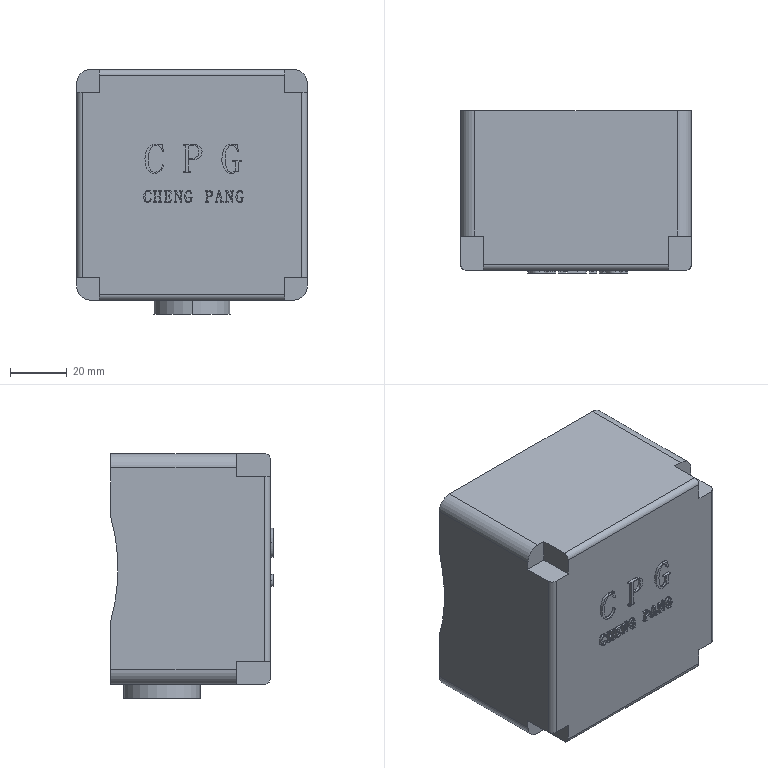Part | SolidWorks | features BaseBody 1 | 1 solid | 327 faces | box 81 x 57 x 86 mm | volume 359652 mm3 | plane 211 | spline 103 | cylinder 13 | commonest cylinder face diameters 4 x4 10 x4 20 x2 27 x2 133 x1